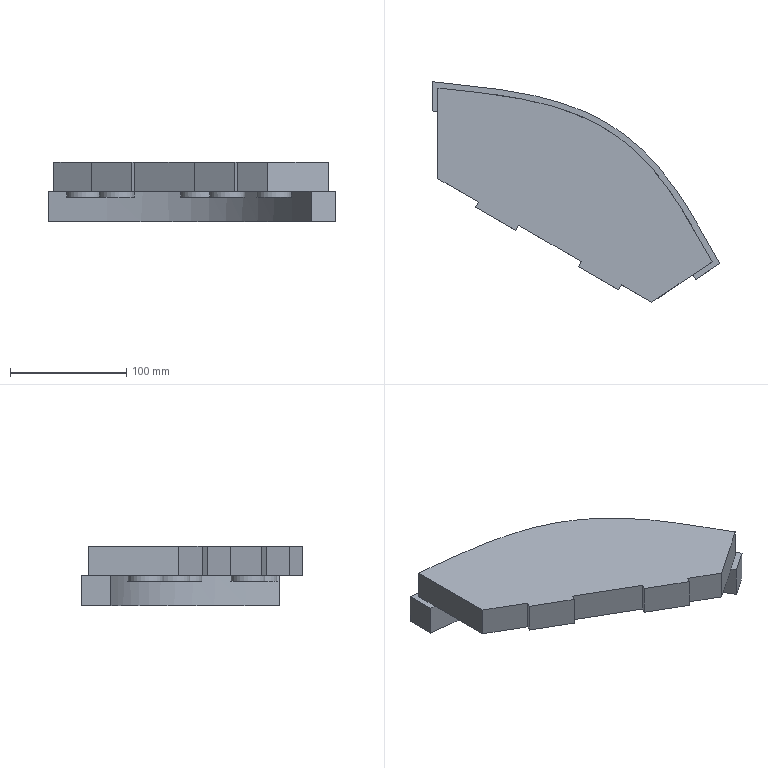Part | NX | features solid 2 | 1 solid | 30 faces | box 247.537 x 189.834 x 51 mm | volume 812442 mm3 | plane 22 | cylinder 5 | spline 3 | commonest cylinder face diameters 30 x5
STEP:
#1=CARTESIAN_POINT('',(-320.,-259.481,20.));
#2=VERTEX_POINT('',#1);
#3=CARTESIAN_POINT('',(-320.,-239.371,20.));
#4=VERTEX_POINT('',#3);
#5=CARTESIAN_POINT('',(-320.,-348.688,20.));
#6=DIRECTION('',(0.,1.,0.));
#7=VECTOR('',#6,1000.);
#8=LINE('',#5,#7);
#9=EDGE_CURVE('',#2,#4,#8,.T.);
#10=ORIENTED_EDGE('',*,*,#9,.T.);
#11=CARTESIAN_POINT('',(-84.106,-388.69,20.));
#12=VERTEX_POINT('',#11);
#13=CARTESIAN_POINT('',(-320.,-239.371,20.));
#14=CARTESIAN_POINT('',(-307.444,-240.685,20.));
#15=CARTESIAN_POINT('',(-282.388,-243.232,20.));
#16=CARTESIAN_POINT('',(-245.249,-248.591,20.));
#17=CARTESIAN_POINT('',(-209.143,-257.743,20.));
#18=CARTESIAN_POINT('',(-175.405,-272.915,20.));
#19=CARTESIAN_POINT('',(-146.181,-295.434,20.));
#20=CARTESIAN_POINT('',(-122.393,-323.908,20.));
#21=CARTESIAN_POINT('',(-102.621,-355.678,20.));
#22=CARTESIAN_POINT('',(-90.362,-377.698,20.));
#23=CARTESIAN_POINT('',(-84.106,-388.69,20.));
#24=B_SPLINE_CURVE_WITH_KNOTS('',3,(#13,#14,#15,#16,#17,#18,#19,#20,#21,#22,#23),.UNSPECIFIED.,.F.,.F.,(4,1,1,1,1,1,1,1,4),(0.01774,0.1387,0.2596,0.3805,0.5015,0.6224,0.7433,0.8643,0.9852),.UNSPECIFIED.);
#25=EDGE_CURVE('',#4,#12,#24,.T.);
#26=ORIENTED_EDGE('',*,*,#25,.T.);
#27=CARTESIAN_POINT('',(-100.733,-399.906,20.));
#28=VERTEX_POINT('',#27);
#29=CARTESIAN_POINT('',(-108.761,-405.32,20.));
#30=DIRECTION('',(-0.829,-0.5592,0.));
#31=VECTOR('',#30,1000.);
#32=LINE('',#29,#31);
#33=EDGE_CURVE('',#12,#28,#32,.T.);
#34=ORIENTED_EDGE('',*,*,#33,.T.);
#35=CARTESIAN_POINT('',(-98.242,-404.256,20.));
#36=VERTEX_POINT('',#35);
#37=CARTESIAN_POINT('',(-325.,-258.957,20.));
#38=CARTESIAN_POINT('',(-316.722,-259.827,20.));
#39=CARTESIAN_POINT('',(-294.324,-262.123,20.));
#40=CARTESIAN_POINT('',(-258.889,-266.42,20.));
#41=CARTESIAN_POINT('',(-226.806,-273.525,20.));
#42=CARTESIAN_POINT('',(-203.149,-282.324,20.));
#43=CARTESIAN_POINT('',(-186.806,-290.617,20.));
#44=CARTESIAN_POINT('',(-171.788,-300.874,20.));
#45=CARTESIAN_POINT('',(-158.202,-313.043,20.));
#46=CARTESIAN_POINT('',(-145.734,-327.185,20.));
#47=CARTESIAN_POINT('',(-130.501,-348.116,20.));
#48=CARTESIAN_POINT('',(-116.6,-371.801,20.));
#49=CARTESIAN_POINT('',(-104.721,-392.924,20.));
#50=CARTESIAN_POINT('',(-99.69,-401.736,20.));
#51=CARTESIAN_POINT('',(-98.242,-404.256,20.));
#52=B_SPLINE_CURVE_WITH_KNOTS('',3,(#37,#38,#39,#40,#41,#42,#43,#44,#45,#46,#47,#48,#49,#50,#51),.UNSPECIFIED.,.F.,.F.,(4,1,1,1,1,1,1,1,1,1,1,1,4),(0.,0.07955,0.2169,0.3543,0.423,0.4917,0.5604,0.6291,0.6978,0.7665,0.9039,0.9726,1.),.UNSPECIFIED.);
#53=EDGE_CURVE('',#36,#28,#52,.F.);
#54=ORIENTED_EDGE('',*,*,#53,.F.);
#55=CARTESIAN_POINT('',(-77.463,-390.241,20.));
#56=VERTEX_POINT('',#55);
#57=CARTESIAN_POINT('',(-98.242,-404.256,20.));
#58=DIRECTION('',(-0.829,-0.5592,0.));
#59=VECTOR('',#58,1000.);
#60=LINE('',#57,#59);
#61=EDGE_CURVE('',#56,#36,#60,.T.);
#62=ORIENTED_EDGE('',*,*,#61,.F.);
#63=CARTESIAN_POINT('',(-325.,-233.817,20.));
#64=VERTEX_POINT('',#63);
#65=CARTESIAN_POINT('',(-325.,-233.817,20.));
#66=CARTESIAN_POINT('',(-317.55,-234.605,20.));
#67=CARTESIAN_POINT('',(-296.291,-236.79,20.));
#68=CARTESIAN_POINT('',(-261.264,-240.795,20.));
#69=CARTESIAN_POINT('',(-220.344,-248.886,20.));
#70=CARTESIAN_POINT('',(-187.701,-261.197,20.));
#71=CARTESIAN_POINT('',(-163.887,-275.581,20.));
#72=CARTESIAN_POINT('',(-147.555,-288.567,20.));
#73=CARTESIAN_POINT('',(-132.971,-303.448,20.));
#74=CARTESIAN_POINT('',(-115.628,-325.186,20.));
#75=CARTESIAN_POINT('',(-97.505,-354.461,20.));
#76=CARTESIAN_POINT('',(-84.207,-378.469,20.));
#77=CARTESIAN_POINT('',(-77.463,-390.241,20.));
#78=B_SPLINE_CURVE_WITH_KNOTS('',3,(#65,#66,#67,#68,#69,#70,#71,#72,#73,#74,#75,#76,#77),.UNSPECIFIED.,.F.,.F.,(4,1,1,1,1,1,1,1,1,1,4),(0.,0.0718,0.2048,0.3379,0.4709,0.5374,0.6039,0.6704,0.7369,0.87,1.),.UNSPECIFIED.);
#79=EDGE_CURVE('',#56,#64,#78,.F.);
#80=ORIENTED_EDGE('',*,*,#79,.T.);
#81=CARTESIAN_POINT('',(-325.,-258.957,20.));
#82=VERTEX_POINT('',#81);
#83=CARTESIAN_POINT('',(-325.,-401.561,20.));
#84=DIRECTION('',(0.,1.,0.));
#85=VECTOR('',#84,1000.);
#86=LINE('',#83,#85);
#87=EDGE_CURVE('',#64,#82,#86,.F.);
#88=ORIENTED_EDGE('',*,*,#87,.T.);
#89=CARTESIAN_POINT('',(-325.,-258.957,20.));
#90=CARTESIAN_POINT('',(-316.722,-259.827,20.));
#91=CARTESIAN_POINT('',(-294.324,-262.123,20.));
#92=CARTESIAN_POINT('',(-258.889,-266.42,20.));
#93=CARTESIAN_POINT('',(-226.806,-273.525,20.));
#94=CARTESIAN_POINT('',(-203.149,-282.324,20.));
#95=CARTESIAN_POINT('',(-186.806,-290.617,20.));
#96=CARTESIAN_POINT('',(-171.788,-300.874,20.));
#97=CARTESIAN_POINT('',(-158.202,-313.043,20.));
#98=CARTESIAN_POINT('',(-145.734,-327.185,20.));
#99=CARTESIAN_POINT('',(-130.501,-348.116,20.));
#100=CARTESIAN_POINT('',(-116.6,-371.801,20.));
#101=CARTESIAN_POINT('',(-104.721,-392.924,20.));
#102=CARTESIAN_POINT('',(-99.69,-401.736,20.));
#103=CARTESIAN_POINT('',(-98.242,-404.256,20.));
#104=B_SPLINE_CURVE_WITH_KNOTS('',3,(#89,#90,#91,#92,#93,#94,#95,#96,#97,#98,#99,#100,#101,#102,#103),.UNSPECIFIED.,.F.,.F.,(4,1,1,1,1,1,1,1,1,1,1,1,4),(0.,0.07955,0.2169,0.3543,0.423,0.4917,0.5604,0.6291,0.6978,0.7665,0.9039,0.9726,1.),.UNSPECIFIED.);
#105=EDGE_CURVE('',#2,#82,#104,.F.);
#106=ORIENTED_EDGE('',*,*,#105,.F.);
#107=EDGE_LOOP('',(#10,#26,#34,#54,#62,#80,#88,#106));
#108=FACE_BOUND('',#107,.T.);
#109=CARTESIAN_POINT('',(-53.05,-401.561,20.));
#110=DIRECTION('',(0.,0.,1.));
#111=DIRECTION('',(1.,0.,0.));
#112=AXIS2_PLACEMENT_3D('',#109,#110,#111);
#113=PLANE('',#112);
#114=ADVANCED_FACE('',(#108),#113,.T.);
#115=CARTESIAN_POINT('',(-145.838,-387.024,20.));
#116=VERTEX_POINT('',#115);
#117=CARTESIAN_POINT('',(-130.838,-387.024,20.));
#118=DIRECTION('',(0.,0.,-1.));
#119=DIRECTION('',(-1.,0.,0.));
#120=AXIS2_PLACEMENT_3D('',#117,#118,#119);
#121=CIRCLE('',#120,15.);
#122=EDGE_CURVE('',#116,#116,#121,.T.);
#123=ORIENTED_EDGE('',*,*,#122,.T.);
#124=EDGE_LOOP('',(#123));
#125=FACE_BOUND('',#124,.T.);
#126=CARTESIAN_POINT('',(-115.838,-387.024,15.));
#127=VERTEX_POINT('',#126);
#128=CARTESIAN_POINT('',(-130.838,-387.024,15.));
#129=DIRECTION('',(0.,0.,1.));
#130=DIRECTION('',(1.,0.,0.));
#131=AXIS2_PLACEMENT_3D('',#128,#129,#130);
#132=CIRCLE('',#131,15.);
#133=EDGE_CURVE('',#127,#127,#132,.T.);
#134=ORIENTED_EDGE('',*,*,#133,.T.);
#135=EDGE_LOOP('',(#134));
#136=FACE_BOUND('',#135,.T.);
#137=CARTESIAN_POINT('',(-130.838,-387.024,20.));
#138=DIRECTION('',(0.,0.,-1.));
#139=DIRECTION('',(-0.866,-0.5,0.));
#140=AXIS2_PLACEMENT_3D('',#137,#138,#139);
#141=CYLINDRICAL_SURFACE('',#140,15.);
#142=ADVANCED_FACE('',(#125,#136),#141,.T.);
#143=CARTESIAN_POINT('',(-185.838,-377.024,20.));
#144=VERTEX_POINT('',#143);
#145=CARTESIAN_POINT('',(-170.838,-377.024,20.));
#146=DIRECTION('',(0.,0.,-1.));
#147=DIRECTION('',(-1.,0.,0.));
#148=AXIS2_PLACEMENT_3D('',#145,#146,#147);
#149=CIRCLE('',#148,15.);
#150=EDGE_CURVE('',#144,#144,#149,.T.);
#151=ORIENTED_EDGE('',*,*,#150,.T.);
#152=EDGE_LOOP('',(#151));
#153=FACE_BOUND('',#152,.T.);
#154=CARTESIAN_POINT('',(-157.848,-369.524,15.));
#155=VERTEX_POINT('',#154);
#156=CARTESIAN_POINT('',(-170.838,-377.024,15.));
#157=DIRECTION('',(0.,0.,-1.));
#158=DIRECTION('',(0.866,0.5,0.));
#159=AXIS2_PLACEMENT_3D('',#156,#157,#158);
#160=CIRCLE('',#159,15.);
#161=EDGE_CURVE('',#155,#155,#160,.T.);
#162=ORIENTED_EDGE('',*,*,#161,.F.);
#163=EDGE_LOOP('',(#162));
#164=FACE_BOUND('',#163,.T.);
#165=CARTESIAN_POINT('',(-170.838,-377.024,20.));
#166=DIRECTION('',(0.,0.,-1.));
#167=DIRECTION('',(-0.866,-0.5,0.));
#168=AXIS2_PLACEMENT_3D('',#165,#166,#167);
#169=CYLINDRICAL_SURFACE('',#168,15.);
#170=ADVANCED_FACE('',(#153,#164),#169,.T.);
#171=CARTESIAN_POINT('',(-325.,-258.957,-6.));
#172=VERTEX_POINT('',#171);
#173=CARTESIAN_POINT('',(-325.,-233.817,-6.));
#174=VERTEX_POINT('',#173);
#175=CARTESIAN_POINT('',(-325.,-258.957,-6.));
#176=DIRECTION('',(0.,1.,0.));
#177=VECTOR('',#176,1000.);
#178=LINE('',#175,#177);
#179=EDGE_CURVE('',#172,#174,#178,.T.);
#180=ORIENTED_EDGE('',*,*,#179,.F.);
#181=CARTESIAN_POINT('',(-325.,-258.957,45.));
#182=DIRECTION('',(0.,0.,-1.));
#183=VECTOR('',#182,1000.);
#184=LINE('',#181,#183);
#185=EDGE_CURVE('',#82,#172,#184,.T.);
#186=ORIENTED_EDGE('',*,*,#185,.F.);
#187=ORIENTED_EDGE('',*,*,#87,.F.);
#188=CARTESIAN_POINT('',(-325.,-233.817,45.));
#189=DIRECTION('',(0.,0.,-1.));
#190=VECTOR('',#189,1000.);
#191=LINE('',#188,#190);
#192=EDGE_CURVE('',#64,#174,#191,.T.);
#193=ORIENTED_EDGE('',*,*,#192,.T.);
#194=EDGE_LOOP('',(#180,#186,#187,#193));
#195=FACE_BOUND('',#194,.T.);
#196=CARTESIAN_POINT('',(-325.,-560.,0.));
#197=DIRECTION('',(1.,0.,0.));
#198=DIRECTION('',(0.,0.,-1.));
#199=AXIS2_PLACEMENT_3D('',#196,#197,#198);
#200=PLANE('',#199);
#201=ADVANCED_FACE('',(#195),#200,.F.);
#202=CARTESIAN_POINT('',(-77.463,-390.241,-6.));
#203=VERTEX_POINT('',#202);
#204=CARTESIAN_POINT('',(-325.,-233.817,-6.));
#205=CARTESIAN_POINT('',(-317.55,-234.605,-6.));
#206=CARTESIAN_POINT('',(-296.291,-236.79,-6.));
#207=CARTESIAN_POINT('',(-261.264,-240.795,-6.));
#208=CARTESIAN_POINT('',(-220.344,-248.886,-6.));
#209=CARTESIAN_POINT('',(-187.701,-261.197,-6.));
#210=CARTESIAN_POINT('',(-163.887,-275.581,-6.));
#211=CARTESIAN_POINT('',(-147.555,-288.567,-6.));
#212=CARTESIAN_POINT('',(-132.971,-303.448,-6.));
#213=CARTESIAN_POINT('',(-115.628,-325.186,-6.));
#214=CARTESIAN_POINT('',(-97.505,-354.461,-6.));
#215=CARTESIAN_POINT('',(-84.207,-378.469,-6.));
#216=CARTESIAN_POINT('',(-77.463,-390.241,-6.));
#217=B_SPLINE_CURVE_WITH_KNOTS('',3,(#204,#205,#206,#207,#208,#209,#210,#211,#212,#213,#214,#215,#216),.UNSPECIFIED.,.F.,.F.,(4,1,1,1,1,1,1,1,1,1,4),(0.,0.0718,0.2048,0.3379,0.4709,0.5374,0.6039,0.6704,0.7369,0.87,1.),.UNSPECIFIED.);
#218=EDGE_CURVE('',#174,#203,#217,.T.);
#219=ORIENTED_EDGE('',*,*,#218,.T.);
#220=CARTESIAN_POINT('',(-98.242,-404.256,-6.));
#221=VERTEX_POINT('',#220);
#222=CARTESIAN_POINT('',(-98.242,-404.256,-6.));
#223=DIRECTION('',(0.829,0.5592,0.));
#224=VECTOR('',#223,1000.);
#225=LINE('',#222,#224);
#226=EDGE_CURVE('',#221,#203,#225,.T.);
#227=ORIENTED_EDGE('',*,*,#226,.F.);
#228=CARTESIAN_POINT('',(-325.,-258.957,-6.));
#229=CARTESIAN_POINT('',(-316.722,-259.827,-6.));
#230=CARTESIAN_POINT('',(-294.324,-262.123,-6.));
#231=CARTESIAN_POINT('',(-258.889,-266.42,-6.));
#232=CARTESIAN_POINT('',(-226.806,-273.525,-6.));
#233=CARTESIAN_POINT('',(-203.149,-282.324,-6.));
#234=CARTESIAN_POINT('',(-186.806,-290.617,-6.));
#235=CARTESIAN_POINT('',(-171.788,-300.874,-6.));
#236=CARTESIAN_POINT('',(-158.202,-313.043,-6.));
#237=CARTESIAN_POINT('',(-145.734,-327.185,-6.));
#238=CARTESIAN_POINT('',(-130.501,-348.116,-6.));
#239=CARTESIAN_POINT('',(-116.6,-371.801,-6.));
#240=CARTESIAN_POINT('',(-104.721,-392.924,-6.));
#241=CARTESIAN_POINT('',(-99.69,-401.736,-6.));
#242=CARTESIAN_POINT('',(-98.242,-404.256,-6.));
#243=B_SPLINE_CURVE_WITH_KNOTS('',3,(#228,#229,#230,#231,#232,#233,#234,#235,#236,#237,#238,#239,#240,#241,#242),.UNSPECIFIED.,.F.,.F.,(4,1,1,1,1,1,1,1,1,1,1,1,4),(0.,0.07955,0.2169,0.3543,0.423,0.4917,0.5604,0.6291,0.6978,0.7665,0.9039,0.9726,1.),.UNSPECIFIED.);
#244=EDGE_CURVE('',#172,#221,#243,.T.);
#245=ORIENTED_EDGE('',*,*,#244,.F.);
#246=ORIENTED_EDGE('',*,*,#179,.T.);
#247=EDGE_LOOP('',(#219,#227,#245,#246));
#248=FACE_BOUND('',#247,.T.);
#249=CARTESIAN_POINT('',(-582.311,-1052.635,-6.));
#250=DIRECTION('',(0.,0.,1.));
#251=DIRECTION('',(1.,0.,0.));
#252=AXIS2_PLACEMENT_3D('',#249,#250,#251);
#253=PLANE('',#252);
#254=ADVANCED_FACE('',(#248),#253,.F.);
#255=CARTESIAN_POINT('',(-280.838,-312.024,20.));
#256=VERTEX_POINT('',#255);
#257=CARTESIAN_POINT('',(-265.838,-312.024,20.));
#258=DIRECTION('',(0.,0.,-1.));
#259=DIRECTION('',(-1.,0.,0.));
#260=AXIS2_PLACEMENT_3D('',#257,#258,#259);
#261=CIRCLE('',#260,15.);
#262=EDGE_CURVE('',#256,#256,#261,.T.);
#263=ORIENTED_EDGE('',*,*,#262,.F.);
#264=EDGE_LOOP('',(#263));
#265=FACE_BOUND('',#264,.T.);
#266=ORIENTED_EDGE('',*,*,#122,.F.);
#267=EDGE_LOOP('',(#266));
#268=FACE_BOUND('',#267,.T.);
#269=CARTESIAN_POINT('',(-309.188,-288.543,20.));
#270=VERTEX_POINT('',#269);
#271=CARTESIAN_POINT('',(-294.188,-288.543,20.));
#272=DIRECTION('',(0.,0.,-1.));
#273=DIRECTION('',(-1.,0.,0.));
#274=AXIS2_PLACEMENT_3D('',#271,#272,#273);
#275=CIRCLE('',#274,15.);
#276=EDGE_CURVE('',#270,#270,#275,.T.);
#277=ORIENTED_EDGE('',*,*,#276,.F.);
#278=EDGE_LOOP('',(#277));
#279=FACE_BOUND('',#278,.T.);
#280=CARTESIAN_POINT('',(-210.838,-322.024,20.));
#281=VERTEX_POINT('',#280);
#282=CARTESIAN_POINT('',(-195.838,-322.024,20.));
#283=DIRECTION('',(0.,0.,-1.));
#284=DIRECTION('',(-1.,0.,0.));
#285=AXIS2_PLACEMENT_3D('',#282,#283,#284);
#286=CIRCLE('',#285,15.);
#287=EDGE_CURVE('',#281,#281,#286,.T.);
#288=ORIENTED_EDGE('',*,*,#287,.F.);
#289=EDGE_LOOP('',(#288));
#290=FACE_BOUND('',#289,.T.);
#291=CARTESIAN_POINT('',(-320.,-259.481,20.));
#292=CARTESIAN_POINT('',(-308.475,-260.684,20.));
#293=CARTESIAN_POINT('',(-285.416,-263.051,20.));
#294=CARTESIAN_POINT('',(-251.082,-267.927,20.));
#295=CARTESIAN_POINT('',(-222.914,-274.771,20.));
#296=CARTESIAN_POINT('',(-201.046,-283.292,20.));
#297=CARTESIAN_POINT('',(-185.448,-291.461,20.));
#298=CARTESIAN_POINT('',(-171.129,-301.443,20.));
#299=CARTESIAN_POINT('',(-154.042,-316.84,20.));
#300=CARTESIAN_POINT('',(-135.792,-339.802,20.));
#301=CARTESIAN_POINT('',(-117.789,-369.539,20.));
#302=CARTESIAN_POINT('',(-106.486,-389.828,20.));
#303=CARTESIAN_POINT('',(-100.733,-399.906,20.));
#304=B_SPLINE_CURVE_WITH_KNOTS('',3,(#291,#292,#293,#294,#295,#296,#297,#298,#299,#300,#301,#302,#303),.UNSPECIFIED.,.F.,.F.,(4,1,1,1,1,1,1,1,1,1,4),(0.6352,0.6699,0.7047,0.7394,0.7568,0.7742,0.7916,0.809,0.8437,0.8785,0.9133),.UNSPECIFIED.);
#305=EDGE_CURVE('',#2,#28,#304,.T.);
#306=ORIENTED_EDGE('',*,*,#305,.T.);
#307=CARTESIAN_POINT('',(-135.938,-423.652,20.));
#308=VERTEX_POINT('',#307);
#309=CARTESIAN_POINT('',(-108.761,-405.32,20.));
#310=DIRECTION('',(-0.829,-0.5592,0.));
#311=VECTOR('',#310,1000.);
#312=LINE('',#309,#311);
#313=EDGE_CURVE('',#28,#308,#312,.T.);
#314=ORIENTED_EDGE('',*,*,#313,.T.);
#315=CARTESIAN_POINT('',(-161.919,-408.652,20.));
#316=VERTEX_POINT('',#315);
#317=CARTESIAN_POINT('',(-229.815,-369.451,20.));
#318=DIRECTION('',(-0.866,0.5,0.));
#319=VECTOR('',#318,1000.);
#320=LINE('',#317,#319);
#321=EDGE_CURVE('',#308,#316,#320,.T.);
#322=ORIENTED_EDGE('',*,*,#321,.T.);
#323=CARTESIAN_POINT('',(-164.419,-412.982,20.));
#324=VERTEX_POINT('',#323);
#325=CARTESIAN_POINT('',(-164.419,-412.982,20.));
#326=DIRECTION('',(0.5,0.866,0.));
#327=VECTOR('',#326,1000.);
#328=LINE('',#325,#327);
#329=EDGE_CURVE('',#324,#316,#328,.T.);
#330=ORIENTED_EDGE('',*,*,#329,.F.);
#331=CARTESIAN_POINT('',(-199.06,-392.982,20.));
#332=VERTEX_POINT('',#331);
#333=CARTESIAN_POINT('',(-108.875,-445.05,20.));
#334=DIRECTION('',(-0.866,0.5,0.));
#335=VECTOR('',#334,1000.);
#336=LINE('',#333,#335);
#337=EDGE_CURVE('',#324,#332,#336,.T.);
#338=ORIENTED_EDGE('',*,*,#337,.T.);
#339=CARTESIAN_POINT('',(-196.56,-388.652,20.));
#340=VERTEX_POINT('',#339);
#341=CARTESIAN_POINT('',(-199.06,-392.982,20.));
#342=DIRECTION('',(0.5,0.866,0.));
#343=VECTOR('',#342,1000.);
#344=LINE('',#341,#343);
#345=EDGE_CURVE('',#332,#340,#344,.T.);
#346=ORIENTED_EDGE('',*,*,#345,.T.);
#347=CARTESIAN_POINT('',(-250.718,-357.383,20.));
#348=VERTEX_POINT('',#347);
#349=CARTESIAN_POINT('',(-229.815,-369.451,20.));
#350=DIRECTION('',(-0.866,0.5,0.));
#351=VECTOR('',#350,1000.);
#352=LINE('',#349,#351);
#353=EDGE_CURVE('',#340,#348,#352,.T.);
#354=ORIENTED_EDGE('',*,*,#353,.T.);
#355=CARTESIAN_POINT('',(-253.218,-361.713,20.));
#356=VERTEX_POINT('',#355);
#357=CARTESIAN_POINT('',(-253.218,-361.713,20.));
#358=DIRECTION('',(-0.5,-0.866,0.));
#359=VECTOR('',#358,1000.);
#360=LINE('',#357,#359);
#361=EDGE_CURVE('',#356,#348,#360,.F.);
#362=ORIENTED_EDGE('',*,*,#361,.F.);
#363=CARTESIAN_POINT('',(-287.859,-341.713,20.));
#364=VERTEX_POINT('',#363);
#365=CARTESIAN_POINT('',(-232.315,-373.782,20.));
#366=DIRECTION('',(-0.866,0.5,0.));
#367=VECTOR('',#366,1000.);
#368=LINE('',#365,#367);
#369=EDGE_CURVE('',#356,#364,#368,.T.);
#370=ORIENTED_EDGE('',*,*,#369,.T.);
#371=CARTESIAN_POINT('',(-285.359,-337.383,20.));
#372=VERTEX_POINT('',#371);
#373=CARTESIAN_POINT('',(-287.859,-341.713,20.));
#374=DIRECTION('',(-0.5,-0.866,0.));
#375=VECTOR('',#374,1000.);
#376=LINE('',#373,#375);
#377=EDGE_CURVE('',#364,#372,#376,.F.);
#378=ORIENTED_EDGE('',*,*,#377,.T.);
#379=CARTESIAN_POINT('',(-320.,-317.383,20.));
#380=VERTEX_POINT('',#379);
#381=CARTESIAN_POINT('',(-229.815,-369.451,20.));
#382=DIRECTION('',(-0.866,0.5,0.));
#383=VECTOR('',#382,1000.);
#384=LINE('',#381,#383);
#385=EDGE_CURVE('',#372,#380,#384,.T.);
#386=ORIENTED_EDGE('',*,*,#385,.T.);
#387=CARTESIAN_POINT('',(-320.,-348.688,20.));
#388=DIRECTION('',(0.,1.,0.));
#389=VECTOR('',#388,1000.);
#390=LINE('',#387,#389);
#391=EDGE_CURVE('',#380,#2,#390,.T.);
#392=ORIENTED_EDGE('',*,*,#391,.T.);
#393=EDGE_LOOP('',(#306,#314,#322,#330,#338,#346,#354,#362,#370,#378,#386,#392));
#394=FACE_BOUND('',#393,.T.);
#395=ORIENTED_EDGE('',*,*,#150,.F.);
#396=EDGE_LOOP('',(#395));
#397=FACE_BOUND('',#396,.T.);
#398=CARTESIAN_POINT('',(-53.05,-401.561,20.));
#399=DIRECTION('',(0.,0.,-1.));
#400=DIRECTION('',(-1.,0.,0.));
#401=AXIS2_PLACEMENT_3D('',#398,#399,#400);
#402=PLANE('',#401);
#403=ADVANCED_FACE('',(#265,#268,#279,#290,#394,#397),#402,.T.);
#404=CARTESIAN_POINT('',(-320.,-317.383,45.));
#405=VERTEX_POINT('',#404);
#406=CARTESIAN_POINT('',(-320.,-239.371,45.));
#407=VERTEX_POINT('',#406);
#408=CARTESIAN_POINT('',(-320.,-348.688,45.));
#409=DIRECTION('',(0.,1.,0.));
#410=VECTOR('',#409,1000.);
#411=LINE('',#408,#410);
#412=EDGE_CURVE('',#405,#407,#411,.T.);
#413=ORIENTED_EDGE('',*,*,#412,.F.);
#414=CARTESIAN_POINT('',(-285.359,-337.383,45.));
#415=VERTEX_POINT('',#414);
#416=CARTESIAN_POINT('',(-131.12,-426.433,45.));
#417=DIRECTION('',(-0.866,0.5,0.));
#418=VECTOR('',#417,1000.);
#419=LINE('',#416,#418);
#420=EDGE_CURVE('',#415,#405,#419,.T.);
#421=ORIENTED_EDGE('',*,*,#420,.F.);
#422=CARTESIAN_POINT('',(-287.859,-341.713,45.));
#423=VERTEX_POINT('',#422);
#424=CARTESIAN_POINT('',(-287.859,-341.713,45.));
#425=DIRECTION('',(0.5,0.866,0.));
#426=VECTOR('',#425,1000.);
#427=LINE('',#424,#426);
#428=EDGE_CURVE('',#423,#415,#427,.T.);
#429=ORIENTED_EDGE('',*,*,#428,.F.);
#430=CARTESIAN_POINT('',(-253.218,-361.713,45.));
#431=VERTEX_POINT('',#430);
#432=CARTESIAN_POINT('',(-133.62,-430.763,45.));
#433=DIRECTION('',(-0.866,0.5,0.));
#434=VECTOR('',#433,1000.);
#435=LINE('',#432,#434);
#436=EDGE_CURVE('',#431,#423,#435,.T.);
#437=ORIENTED_EDGE('',*,*,#436,.F.);
#438=CARTESIAN_POINT('',(-250.718,-357.383,45.));
#439=VERTEX_POINT('',#438);
#440=CARTESIAN_POINT('',(-253.218,-361.713,45.));
#441=DIRECTION('',(0.5,0.866,0.));
#442=VECTOR('',#441,1000.);
#443=LINE('',#440,#442);
#444=EDGE_CURVE('',#431,#439,#443,.T.);
#445=ORIENTED_EDGE('',*,*,#444,.T.);
#446=CARTESIAN_POINT('',(-196.56,-388.652,45.));
#447=VERTEX_POINT('',#446);
#448=CARTESIAN_POINT('',(-131.12,-426.433,45.));
#449=DIRECTION('',(-0.866,0.5,0.));
#450=VECTOR('',#449,1000.);
#451=LINE('',#448,#450);
#452=EDGE_CURVE('',#447,#439,#451,.T.);
#453=ORIENTED_EDGE('',*,*,#452,.F.);
#454=CARTESIAN_POINT('',(-199.06,-392.982,45.));
#455=VERTEX_POINT('',#454);
#456=CARTESIAN_POINT('',(-199.06,-392.982,45.));
#457=DIRECTION('',(0.5,0.866,0.));
#458=VECTOR('',#457,1000.);
#459=LINE('',#456,#458);
#460=EDGE_CURVE('',#455,#447,#459,.T.);
#461=ORIENTED_EDGE('',*,*,#460,.F.);
#462=CARTESIAN_POINT('',(-164.419,-412.982,45.));
#463=VERTEX_POINT('',#462);
#464=CARTESIAN_POINT('',(-10.18,-502.032,45.));
#465=DIRECTION('',(-0.866,0.5,0.));
#466=VECTOR('',#465,1000.);
#467=LINE('',#464,#466);
#468=EDGE_CURVE('',#463,#455,#467,.T.);
#469=ORIENTED_EDGE('',*,*,#468,.F.);
#470=CARTESIAN_POINT('',(-161.919,-408.652,45.));
#471=VERTEX_POINT('',#470);
#472=CARTESIAN_POINT('',(-164.419,-412.982,45.));
#473=DIRECTION('',(0.5,0.866,0.));
#474=VECTOR('',#473,1000.);
#475=LINE('',#472,#474);
#476=EDGE_CURVE('',#463,#471,#475,.T.);
#477=ORIENTED_EDGE('',*,*,#476,.T.);
#478=CARTESIAN_POINT('',(-135.938,-423.652,45.));
#479=VERTEX_POINT('',#478);
#480=CARTESIAN_POINT('',(-131.12,-426.433,45.));
#481=DIRECTION('',(-0.866,0.5,0.));
#482=VECTOR('',#481,1000.);
#483=LINE('',#480,#482);
#484=EDGE_CURVE('',#479,#471,#483,.T.);
#485=ORIENTED_EDGE('',*,*,#484,.F.);
#486=CARTESIAN_POINT('',(-84.106,-388.69,45.));
#487=VERTEX_POINT('',#486);
#488=CARTESIAN_POINT('',(-108.761,-405.32,45.));
#489=DIRECTION('',(-0.829,-0.5592,0.));
#490=VECTOR('',#489,1000.);
#491=LINE('',#488,#490);
#492=EDGE_CURVE('',#487,#479,#491,.T.);
#493=ORIENTED_EDGE('',*,*,#492,.F.);
#494=CARTESIAN_POINT('',(-84.106,-388.69,45.));
#495=CARTESIAN_POINT('',(-85.647,-385.982,45.));
#496=CARTESIAN_POINT('',(-88.727,-380.563,45.));
#497=CARTESIAN_POINT('',(-92.552,-373.785,45.));
#498=CARTESIAN_POINT('',(-95.629,-368.349,45.));
#499=CARTESIAN_POINT('',(-97.957,-364.289,45.));
#500=CARTESIAN_POINT('',(-99.9,-360.932,45.));
#501=CARTESIAN_POINT('',(-101.482,-358.221,45.));
#502=CARTESIAN_POINT('',(-102.617,-356.285,45.));
#503=CARTESIAN_POINT('',(-103.968,-353.996,45.));
#504=CARTESIAN_POINT('',(-105.653,-351.166,45.));
#505=CARTESIAN_POINT('',(-107.726,-347.73,45.));
#506=CARTESIAN_POINT('',(-109.714,-344.499,45.));
#507=CARTESIAN_POINT('',(-111.054,-342.356,45.));
#508=CARTESIAN_POINT('',(-111.826,-341.133,45.));
#509=CARTESIAN_POINT('',(-112.348,-340.31,45.));
#510=CARTESIAN_POINT('',(-113.056,-339.2,45.));
#511=CARTESIAN_POINT('',(-113.932,-337.837,45.));
#512=CARTESIAN_POINT('',(-115.49,-335.441,45.));
#513=CARTESIAN_POINT('',(-117.678,-332.15,45.));
#514=CARTESIAN_POINT('',(-119.851,-328.982,45.));
#515=CARTESIAN_POINT('',(-121.348,-326.852,45.));
#516=CARTESIAN_POINT('',(-122.214,-325.635,45.));
#517=CARTESIAN_POINT('',(-122.82,-324.791,45.));
#518=CARTESIAN_POINT('',(-123.584,-323.737,45.));
#519=CARTESIAN_POINT('',(-124.55,-322.418,45.));
#520=CARTESIAN_POINT('',(-126.27,-320.104,45.));
#521=CARTESIAN_POINT('',(-128.729,-316.899,45.));
#522=CARTESIAN_POINT('',(-131.71,-313.175,45.));
#523=CARTESIAN_POINT('',(-135.713,-308.387,45.));
#524=CARTESIAN_POINT('',(-139.769,-303.854,45.));
#525=CARTESIAN_POINT('',(-143.344,-300.132,45.));
#526=CARTESIAN_POINT('',(-145.423,-298.047,45.));
#527=CARTESIAN_POINT('',(-146.92,-296.581,45.));
#528=CARTESIAN_POINT('',(-148.681,-294.902,45.));
#529=CARTESIAN_POINT('',(-150.968,-292.786,45.));
#530=CARTESIAN_POINT('',(-155.076,-289.142,45.));
#531=CARTESIAN_POINT('',(-161.107,-284.243,45.));
#532=CARTESIAN_POINT('',(-167.411,-279.706,45.));
#533=CARTESIAN_POINT('',(-172.571,-276.323,45.));
#534=CARTESIAN_POINT('',(-176.604,-273.848,45.));
#535=CARTESIAN_POINT('',(-180.375,-271.68,45.));
#536=CARTESIAN_POINT('',(-185.668,-268.822,45.));
#537=CARTESIAN_POINT('',(-192.496,-265.486,45.));
#538=CARTESIAN_POINT('',(-199.688,-262.414,45.));
#539=CARTESIAN_POINT('',(-204.89,-260.415,45.));
#540=CARTESIAN_POINT('',(-207.551,-259.447,45.));
#541=CARTESIAN_POINT('',(-209.061,-258.912,45.));
#542=CARTESIAN_POINT('',(-210.265,-258.493,45.));
#543=CARTESIAN_POINT('',(-211.229,-258.164,45.));
#544=CARTESIAN_POINT('',(-212.61,-257.7,45.));
#545=CARTESIAN_POINT('',(-215.012,-256.913,45.));
#546=CARTESIAN_POINT('',(-219.945,-255.377,45.));
#547=CARTESIAN_POINT('',(-225.8,-253.731,45.));
#548=CARTESIAN_POINT('',(-231.888,-252.19,45.));
#549=CARTESIAN_POINT('',(-236.572,-251.087,45.));
#550=CARTESIAN_POINT('',(-240.558,-250.215,45.));
#551=CARTESIAN_POINT('',(-243.425,-249.623,45.));
#552=CARTESIAN_POINT('',(-245.035,-249.299,45.));
#553=CARTESIAN_POINT('',(-246.369,-249.037,45.));
#554=CARTESIAN_POINT('',(-247.258,-248.865,45.));
#555=CARTESIAN_POINT('',(-248.616,-248.606,45.));
#556=CARTESIAN_POINT('',(-250.955,-248.17,45.));
#557=CARTESIAN_POINT('',(-254.441,-247.55,45.));
#558=CARTESIAN_POINT('',(-258.776,-246.824,45.));
#559=CARTESIAN_POINT('',(-263.283,-246.113,45.));
#560=CARTESIAN_POINT('',(-267.958,-245.416,45.));
#561=CARTESIAN_POINT('',(-271.994,-244.849,45.));
#562=CARTESIAN_POINT('',(-275.306,-244.402,45.));
#563=CARTESIAN_POINT('',(-277.835,-244.071,45.));
#564=CARTESIAN_POINT('',(-279.969,-243.799,45.));
#565=CARTESIAN_POINT('',(-281.498,-243.608,45.));
#566=CARTESIAN_POINT('',(-282.35,-243.502,45.));
#567=CARTESIAN_POINT('',(-283.068,-243.414,45.));
#568=CARTESIAN_POINT('',(-283.497,-243.362,45.));
#569=CARTESIAN_POINT('',(-284.179,-243.279,45.));
#570=CARTESIAN_POINT('',(-285.345,-243.139,45.));
#571=CARTESIAN_POINT('',(-287.787,-242.849,45.));
#572=CARTESIAN_POINT('',(-290.744,-242.507,45.));
#573=CARTESIAN_POINT('',(-293.883,-242.153,45.));
#574=CARTESIAN_POINT('',(-295.92,-241.927,45.));
#575=CARTESIAN_POINT('',(-297.593,-241.742,45.));
#576=CARTESIAN_POINT('',(-298.874,-241.603,45.));
#577=CARTESIAN_POINT('',(-299.948,-241.486,45.));
#578=CARTESIAN_POINT('',(-300.732,-241.401,45.));
#579=CARTESIAN_POINT('',(-301.149,-241.356,45.));
#580=CARTESIAN_POINT('',(-301.559,-241.312,45.));
#581=CARTESIAN_POINT('',(-301.604,-241.307,45.));
#582=CARTESIAN_POINT('',(-301.8,-241.286,45.));
#583=CARTESIAN_POINT('',(-302.102,-241.254,45.));
#584=CARTESIAN_POINT('',(-302.617,-241.199,45.));
#585=CARTESIAN_POINT('',(-303.307,-241.126,45.));
#586=CARTESIAN_POINT('',(-304.343,-241.016,45.));
#587=CARTESIAN_POINT('',(-305.848,-240.857,45.));
#588=CARTESIAN_POINT('',(-308.707,-240.555,45.));
#589=CARTESIAN_POINT('',(-313.124,-240.091,45.));
#590=CARTESIAN_POINT('',(-317.558,-239.626,45.));
#591=CARTESIAN_POINT('',(-320.,-239.371,45.));
#592=B_SPLINE_CURVE_WITH_KNOTS('',3,(#494,#495,#496,#497,#498,#499,#500,#501,#502,#503,#504,#505,#506,#507,#508,#509,#510,#511,#512,#513,#514,#515,#516,#517,#518,#519,#520,#521,#522,#523,#524,#525,#526,#527,#528,#529,#530,#531,#532,#533,#534,#535,#536,#537,#538,#539,#540,#541,#542,#543,#544,#545,#546,#547,#548,#549,#550,#551,#552,#553,#554,#555,#556,#557,#558,#559,#560,#561,#562,#563,#564,#565,#566,#567,#568,#569,#570,#571,#572,#573,#574,#575,#576,#577,#578,#579,#580,#581,#582,#583,#584,#585,#586,#587,#588,#589,#590,#591),.UNSPECIFIED.,.F.,.F.,(4,1,1,1,1,1,1,1,1,1,1,1,1,1,1,1,1,1,1,1,1,1,1,1,1,1,1,1,1,1,1,1,1,1,1,1,1,1,1,1,1,1,1,1,1,1,1,1,1,1,1,1,1,1,1,1,1,1,1,1,1,1,1,1,1,1,1,1,1,1,1,1,1,1,1,1,1,1,1,1,1,1,1,1,1,1,1,1,1,1,1,1,1,1,1,4),(0.,0.03125,0.0625,0.07812,0.09375,0.1094,0.1172,0.125,0.1328,0.1406,0.1562,0.1719,0.1797,0.1836,0.1875,0.1914,0.1953,0.2031,0.2188,0.2344,0.2422,0.2461,0.25,0.2539,0.2578,0.2656,0.2812,0.2969,0.3125,0.3438,0.3594,0.3672,0.375,0.3828,0.3906,0.4062,0.4375,0.4688,0.4844,0.5,0.5156,0.5312,0.5625,0.5938,0.6094,0.6172,0.6211,0.625,0.6289,0.6328,0.6406,0.6562,0.6875,0.7031,0.7188,0.7344,0.7422,0.7461,0.75,0.7539,0.7578,0.7656,0.7812,0.7969,0.8125,0.8281,0.8438,0.8516,0.8594,0.8672,0.8711,0.873,0.875,0.877,0.8789,0.8828,0.8906,0.9062,0.9141,0.9219,0.9258,0.9297,0.9336,0.9355,0.9365,0.9375,0.9385,0.9395,0.9414,0.9453,0.9492,0.9531,0.9609,0.9688,0.9844,1.),.UNSPECIFIED.);
#593=EDGE_CURVE('',#487,#407,#592,.T.);
#594=ORIENTED_EDGE('',*,*,#593,.T.);
#595=EDGE_LOOP('',(#413,#421,#429,#437,#445,#453,#461,#469,#477,#485,#493,#594));
#596=FACE_BOUND('',#595,.T.);
#597=CARTESIAN_POINT('',(-582.311,-1052.635,45.));
#598=DIRECTION('',(0.,0.,1.));
#599=DIRECTION('',(1.,0.,0.));
#600=AXIS2_PLACEMENT_3D('',#597,#598,#599);
#601=PLANE('',#600);
#602=ADVANCED_FACE('',(#596),#601,.T.);
#603=ORIENTED_EDGE('',*,*,#133,.F.);
#604=EDGE_LOOP('',(#603));
#605=FACE_BOUND('',#604,.T.);
#606=CARTESIAN_POINT('',(-118.429,-400.345,15.));
#607=DIRECTION('',(0.,0.,1.));
#608=DIRECTION('',(1.,0.,0.));
#609=AXIS2_PLACEMENT_3D('',#606,#607,#608);
#610=PLANE('',#609);
#611=ADVANCED_FACE('',(#605),#610,.F.);
#612=ORIENTED_EDGE('',*,*,#391,.F.);
#613=CARTESIAN_POINT('',(-320.,-317.383,45.));
#614=DIRECTION('',(0.,0.,1.));
#615=VECTOR('',#614,1000.);
#616=LINE('',#613,#615);
#617=EDGE_CURVE('',#380,#405,#616,.T.);
#618=ORIENTED_EDGE('',*,*,#617,.T.);
#619=ORIENTED_EDGE('',*,*,#412,.T.);
#620=CARTESIAN_POINT('',(-320.,-239.371,32.5));
#621=DIRECTION('',(0.,0.,1.));
#622=VECTOR('',#621,1000.);
#623=LINE('',#620,#622);
#624=EDGE_CURVE('',#4,#407,#623,.T.);
#625=ORIENTED_EDGE('',*,*,#624,.F.);
#626=ORIENTED_EDGE('',*,*,#9,.F.);
#627=EDGE_LOOP('',(#612,#618,#619,#625,#626));
#628=FACE_BOUND('',#627,.T.);
#629=CARTESIAN_POINT('',(-320.,-348.688,45.));
#630=DIRECTION('',(-1.,0.,0.));
#631=DIRECTION('',(0.,0.,1.));
#632=AXIS2_PLACEMENT_3D('',#629,#630,#631);
#633=PLANE('',#632);
#634=ADVANCED_FACE('',(#628),#633,.T.);
#635=CARTESIAN_POINT('',(-250.838,-312.024,15.));
#636=VERTEX_POINT('',#635);
#637=CARTESIAN_POINT('',(-265.838,-312.024,15.));
#638=DIRECTION('',(0.,0.,1.));
#639=DIRECTION('',(1.,0.,0.));
#640=AXIS2_PLACEMENT_3D('',#637,#638,#639);
#641=CIRCLE('',#640,15.);
#642=EDGE_CURVE('',#636,#636,#641,.T.);
#643=ORIENTED_EDGE('',*,*,#642,.F.);
#644=EDGE_LOOP('',(#643));
#645=FACE_BOUND('',#644,.T.);
#646=CARTESIAN_POINT('',(-258.429,-320.345,15.));
#647=DIRECTION('',(0.,0.,1.));
#648=DIRECTION('',(1.,0.,0.));
#649=AXIS2_PLACEMENT_3D('',#646,#647,#648);
#650=PLANE('',#649);
#651=ADVANCED_FACE('',(#645),#650,.F.);
#652=CARTESIAN_POINT('',(-281.197,-281.043,15.));
#653=VERTEX_POINT('',#652);
#654=CARTESIAN_POINT('',(-294.188,-288.543,15.));
#655=DIRECTION('',(0.,0.,-1.));
#656=DIRECTION('',(0.866,0.5,0.));
#657=AXIS2_PLACEMENT_3D('',#654,#655,#656);
#658=CIRCLE('',#657,15.);
#659=EDGE_CURVE('',#653,#653,#658,.T.);
#660=ORIENTED_EDGE('',*,*,#659,.T.);
#661=EDGE_LOOP('',(#660));
#662=FACE_BOUND('',#661,.T.);
#663=CARTESIAN_POINT('',(-283.429,-300.345,15.));
#664=DIRECTION('',(0.,0.,1.));
#665=DIRECTION('',(1.,0.,0.));
#666=AXIS2_PLACEMENT_3D('',#663,#664,#665);
#667=PLANE('',#666);
#668=ADVANCED_FACE('',(#662),#667,.F.);
#669=ORIENTED_EDGE('',*,*,#161,.T.);
#670=EDGE_LOOP('',(#669));
#671=FACE_BOUND('',#670,.T.);
#672=CARTESIAN_POINT('',(-153.429,-395.345,15.));
#673=DIRECTION('',(0.,0.,1.));
#674=DIRECTION('',(1.,0.,0.));
#675=AXIS2_PLACEMENT_3D('',#672,#673,#674);
#676=PLANE('',#675);
#677=ADVANCED_FACE('',(#671),#676,.F.);
#678=ORIENTED_EDGE('',*,*,#262,.T.);
#679=EDGE_LOOP('',(#678));
#680=FACE_BOUND('',#679,.T.);
#681=ORIENTED_EDGE('',*,*,#642,.T.);
#682=EDGE_LOOP('',(#681));
#683=FACE_BOUND('',#682,.T.);
#684=CARTESIAN_POINT('',(-265.838,-312.024,20.));
#685=DIRECTION('',(0.,0.,-1.));
#686=DIRECTION('',(-0.866,-0.5,0.));
#687=AXIS2_PLACEMENT_3D('',#684,#685,#686);
#688=CYLINDRICAL_SURFACE('',#687,15.);
#689=ADVANCED_FACE('',(#680,#683),#688,.T.);
#690=CARTESIAN_POINT('',(-182.848,-314.524,15.));
#691=VERTEX_POINT('',#690);
#692=CARTESIAN_POINT('',(-195.838,-322.024,15.));
#693=DIRECTION('',(0.,0.,-1.));
#694=DIRECTION('',(0.866,0.5,0.));
#695=AXIS2_PLACEMENT_3D('',#692,#693,#694);
#696=CIRCLE('',#695,15.);
#697=EDGE_CURVE('',#691,#691,#696,.T.);
#698=ORIENTED_EDGE('',*,*,#697,.T.);
#699=EDGE_LOOP('',(#698));
#700=FACE_BOUND('',#699,.T.);
#701=CARTESIAN_POINT('',(-195.838,-322.024,15.));
#702=DIRECTION('',(0.,0.,-1.));
#703=DIRECTION('',(-0.866,-0.5,0.));
#704=AXIS2_PLACEMENT_3D('',#701,#702,#703);
#705=PLANE('',#704);
#706=ADVANCED_FACE('',(#700),#705,.T.);
#707=ORIENTED_EDGE('',*,*,#244,.T.);
#708=CARTESIAN_POINT('',(-98.242,-404.256,45.));
#709=DIRECTION('',(0.,0.,-1.));
#710=VECTOR('',#709,1000.);
#711=LINE('',#708,#710);
#712=EDGE_CURVE('',#36,#221,#711,.T.);
#713=ORIENTED_EDGE('',*,*,#712,.F.);
#714=ORIENTED_EDGE('',*,*,#53,.T.);
#715=ORIENTED_EDGE('',*,*,#305,.F.);
#716=ORIENTED_EDGE('',*,*,#105,.T.);
#717=ORIENTED_EDGE('',*,*,#185,.T.);
#718=EDGE_LOOP('',(#707,#713,#714,#715,#716,#717));
#719=FACE_BOUND('',#718,.T.);
#720=CARTESIAN_POINT('',(-325.,-258.957,20.));
#721=CARTESIAN_POINT('',(-325.,-258.957,-6.));
#722=CARTESIAN_POINT('',(-298.986,-261.69,20.));
#723=CARTESIAN_POINT('',(-298.986,-261.69,-6.));
#724=CARTESIAN_POINT('',(-260.913,-265.249,20.));
#725=CARTESIAN_POINT('',(-260.913,-265.249,-6.));
#726=CARTESIAN_POINT('',(-214.978,-276.918,20.));
#727=CARTESIAN_POINT('',(-214.978,-276.918,-6.));
#728=CARTESIAN_POINT('',(-184.347,-291.007,20.));
#729=CARTESIAN_POINT('',(-184.347,-291.007,-6.));
#730=CARTESIAN_POINT('',(-158.497,-311.525,20.));
#731=CARTESIAN_POINT('',(-158.497,-311.525,-6.));
#732=CARTESIAN_POINT('',(-136.666,-338.441,20.));
#733=CARTESIAN_POINT('',(-136.666,-338.441,-6.));
#734=CARTESIAN_POINT('',(-117.445,-370.042,20.));
#735=CARTESIAN_POINT('',(-117.445,-370.042,-6.));
#736=CARTESIAN_POINT('',(-104.839,-392.778,20.));
#737=CARTESIAN_POINT('',(-104.839,-392.778,-6.));
#738=CARTESIAN_POINT('',(-98.242,-404.256,20.));
#739=CARTESIAN_POINT('',(-98.242,-404.256,-6.));
#740=B_SPLINE_SURFACE_WITH_KNOTS('',3,1,((#720,#721),(#722,#723),(#724,#725),(#726,#727),(#728,#729),(#730,#731),(#732,#733),(#734,#735),(#736,#737),(#738,#739)),.SURF_OF_LINEAR_EXTRUSION.,.F.,.F.,.F.,(4,1,1,1,1,1,1,4),(2,2),(0.,0.25,0.375,0.5,0.625,0.75,0.875,1.),(0.,1.),.UNSPECIFIED.);
#741=ADVANCED_FACE('',(#719),#740,.F.);
#742=ORIENTED_EDGE('',*,*,#659,.F.);
#743=EDGE_LOOP('',(#742));
#744=FACE_BOUND('',#743,.T.);
#745=ORIENTED_EDGE('',*,*,#276,.T.);
#746=EDGE_LOOP('',(#745));
#747=FACE_BOUND('',#746,.T.);
#748=CARTESIAN_POINT('',(-294.188,-288.543,20.));
#749=DIRECTION('',(0.,0.,-1.));
#750=DIRECTION('',(-0.866,-0.5,0.));
#751=AXIS2_PLACEMENT_3D('',#748,#749,#750);
#752=CYLINDRICAL_SURFACE('',#751,15.);
#753=ADVANCED_FACE('',(#744,#747),#752,.T.);
#754=ORIENTED_EDGE('',*,*,#697,.F.);
#755=EDGE_LOOP('',(#754));
#756=FACE_BOUND('',#755,.T.);
#757=ORIENTED_EDGE('',*,*,#287,.T.);
#758=EDGE_LOOP('',(#757));
#759=FACE_BOUND('',#758,.T.);
#760=CARTESIAN_POINT('',(-195.838,-322.024,20.));
#761=DIRECTION('',(0.,0.,-1.));
#762=DIRECTION('',(-0.866,-0.5,0.));
#763=AXIS2_PLACEMENT_3D('',#760,#761,#762);
#764=CYLINDRICAL_SURFACE('',#763,15.);
#765=ADVANCED_FACE('',(#756,#759),#764,.T.);
#766=ORIENTED_EDGE('',*,*,#25,.F.);
#767=ORIENTED_EDGE('',*,*,#624,.T.);
#768=ORIENTED_EDGE('',*,*,#593,.F.);
#769=CARTESIAN_POINT('',(-84.106,-388.69,32.5));
#770=DIRECTION('',(0.,0.,1.));
#771=VECTOR('',#770,1000.);
#772=LINE('',#769,#771);
#773=EDGE_CURVE('',#12,#487,#772,.T.);
#774=ORIENTED_EDGE('',*,*,#773,.F.);
#775=EDGE_LOOP('',(#766,#767,#768,#774));
#776=FACE_BOUND('',#775,.T.);
#777=CARTESIAN_POINT('',(-320.,-239.371,20.));
#778=CARTESIAN_POINT('',(-320.,-239.371,45.));
#779=CARTESIAN_POINT('',(-307.444,-240.685,20.));
#780=CARTESIAN_POINT('',(-307.444,-240.685,45.));
#781=CARTESIAN_POINT('',(-282.388,-243.232,20.));
#782=CARTESIAN_POINT('',(-282.388,-243.232,45.));
#783=CARTESIAN_POINT('',(-245.249,-248.591,20.));
#784=CARTESIAN_POINT('',(-245.249,-248.591,45.));
#785=CARTESIAN_POINT('',(-209.143,-257.743,20.));
#786=CARTESIAN_POINT('',(-209.143,-257.743,45.));
#787=CARTESIAN_POINT('',(-175.405,-272.915,20.));
#788=CARTESIAN_POINT('',(-175.405,-272.915,45.));
#789=CARTESIAN_POINT('',(-146.181,-295.434,20.));
#790=CARTESIAN_POINT('',(-146.181,-295.434,45.));
#791=CARTESIAN_POINT('',(-122.393,-323.908,20.));
#792=CARTESIAN_POINT('',(-122.393,-323.908,45.));
#793=CARTESIAN_POINT('',(-102.621,-355.678,20.));
#794=CARTESIAN_POINT('',(-102.621,-355.678,45.));
#795=CARTESIAN_POINT('',(-90.362,-377.698,20.));
#796=CARTESIAN_POINT('',(-90.362,-377.698,45.));
#797=CARTESIAN_POINT('',(-84.106,-388.69,20.));
#798=CARTESIAN_POINT('',(-84.106,-388.69,45.));
#799=B_SPLINE_SURFACE_WITH_KNOTS('',3,1,((#777,#778),(#779,#780),(#781,#782),(#783,#784),(#785,#786),(#787,#788),(#789,#790),(#791,#792),(#793,#794),(#795,#796),(#797,#798)),.SURF_OF_LINEAR_EXTRUSION.,.F.,.F.,.F.,(4,1,1,1,1,1,1,1,4),(2,2),(0.01774,0.1387,0.2596,0.3805,0.5015,0.6224,0.7433,0.8643,0.9852),(0.,1.),.UNSPECIFIED.);
#800=ADVANCED_FACE('',(#776),#799,.F.);
#801=ORIENTED_EDGE('',*,*,#61,.T.);
#802=ORIENTED_EDGE('',*,*,#712,.T.);
#803=ORIENTED_EDGE('',*,*,#226,.T.);
#804=CARTESIAN_POINT('',(-77.463,-390.241,45.));
#805=DIRECTION('',(0.,0.,-1.));
#806=VECTOR('',#805,1000.);
#807=LINE('',#804,#806);
#808=EDGE_CURVE('',#56,#203,#807,.T.);
#809=ORIENTED_EDGE('',*,*,#808,.F.);
#810=EDGE_LOOP('',(#801,#802,#803,#809));
#811=FACE_BOUND('',#810,.T.);
#812=CARTESIAN_POINT('',(-131.12,-426.433,45.));
#813=DIRECTION('',(-0.5592,0.829,0.));
#814=DIRECTION('',(-0.829,-0.5592,0.));
#815=AXIS2_PLACEMENT_3D('',#812,#813,#814);
#816=PLANE('',#815);
#817=ADVANCED_FACE('',(#811),#816,.F.);
#818=ORIENTED_EDGE('',*,*,#218,.F.);
#819=ORIENTED_EDGE('',*,*,#192,.F.);
#820=ORIENTED_EDGE('',*,*,#79,.F.);
#821=ORIENTED_EDGE('',*,*,#808,.T.);
#822=EDGE_LOOP('',(#818,#819,#820,#821));
#823=FACE_BOUND('',#822,.T.);
#824=CARTESIAN_POINT('',(-325.,-233.817,20.));
#825=CARTESIAN_POINT('',(-325.,-233.817,-6.));
#826=CARTESIAN_POINT('',(-312.031,-235.189,20.));
#827=CARTESIAN_POINT('',(-312.031,-235.189,-6.));
#828=CARTESIAN_POINT('',(-286.074,-237.776,20.));
#829=CARTESIAN_POINT('',(-286.074,-237.776,-6.));
#830=CARTESIAN_POINT('',(-247.289,-243.088,20.));
#831=CARTESIAN_POINT('',(-247.289,-243.088,-6.));
#832=CARTESIAN_POINT('',(-209.18,-252.359,20.));
#833=CARTESIAN_POINT('',(-209.18,-252.359,-6.));
#834=CARTESIAN_POINT('',(-173.183,-268.243,20.));
#835=CARTESIAN_POINT('',(-173.183,-268.243,-6.));
#836=CARTESIAN_POINT('',(-141.991,-292.35,20.));
#837=CARTESIAN_POINT('',(-141.991,-292.35,-6.));
#838=CARTESIAN_POINT('',(-117.044,-322.717,20.));
#839=CARTESIAN_POINT('',(-117.044,-322.717,-6.));
#840=CARTESIAN_POINT('',(-96.6,-356.117,20.));
#841=CARTESIAN_POINT('',(-96.6,-356.117,-6.));
#842=CARTESIAN_POINT('',(-83.946,-378.925,20.));
#843=CARTESIAN_POINT('',(-83.946,-378.925,-6.));
#844=CARTESIAN_POINT('',(-77.463,-390.241,20.));
#845=CARTESIAN_POINT('',(-77.463,-390.241,-6.));
#846=B_SPLINE_SURFACE_WITH_KNOTS('',3,1,((#824,#825),(#826,#827),(#828,#829),(#830,#831),(#832,#833),(#834,#835),(#836,#837),(#838,#839),(#840,#841),(#842,#843),(#844,#845)),.SURF_OF_LINEAR_EXTRUSION.,.F.,.F.,.F.,(4,1,1,1,1,1,1,1,4),(2,2),(0.,0.125,0.25,0.375,0.5,0.625,0.75,0.875,1.),(0.,1.),.UNSPECIFIED.);
#847=ADVANCED_FACE('',(#823),#846,.T.);
#848=ORIENTED_EDGE('',*,*,#484,.T.);
#849=CARTESIAN_POINT('',(-161.919,-408.652,45.));
#850=DIRECTION('',(0.,0.,1.));
#851=VECTOR('',#850,1000.);
#852=LINE('',#849,#851);
#853=EDGE_CURVE('',#316,#471,#852,.T.);
#854=ORIENTED_EDGE('',*,*,#853,.F.);
#855=ORIENTED_EDGE('',*,*,#321,.F.);
#856=CARTESIAN_POINT('',(-135.938,-423.652,45.));
#857=DIRECTION('',(0.,0.,1.));
#858=VECTOR('',#857,1000.);
#859=LINE('',#856,#858);
#860=EDGE_CURVE('',#308,#479,#859,.T.);
#861=ORIENTED_EDGE('',*,*,#860,.T.);
#862=EDGE_LOOP('',(#848,#854,#855,#861));
#863=FACE_BOUND('',#862,.T.);
#864=CARTESIAN_POINT('',(-131.12,-426.433,45.));
#865=DIRECTION('',(-0.5,-0.866,0.));
#866=DIRECTION('',(0.866,-0.5,0.));
#867=AXIS2_PLACEMENT_3D('',#864,#865,#866);
#868=PLANE('',#867);
#869=ADVANCED_FACE('',(#863),#868,.T.);
#870=CARTESIAN_POINT('',(-196.56,-388.652,45.));
#871=DIRECTION('',(0.,0.,1.));
#872=VECTOR('',#871,1000.);
#873=LINE('',#870,#872);
#874=EDGE_CURVE('',#340,#447,#873,.T.);
#875=ORIENTED_EDGE('',*,*,#874,.T.);
#876=ORIENTED_EDGE('',*,*,#452,.T.);
#877=CARTESIAN_POINT('',(-250.718,-357.383,45.));
#878=DIRECTION('',(0.,0.,1.));
#879=VECTOR('',#878,1000.);
#880=LINE('',#877,#879);
#881=EDGE_CURVE('',#348,#439,#880,.T.);
#882=ORIENTED_EDGE('',*,*,#881,.F.);
#883=ORIENTED_EDGE('',*,*,#353,.F.);
#884=EDGE_LOOP('',(#875,#876,#882,#883));
#885=FACE_BOUND('',#884,.T.);
#886=CARTESIAN_POINT('',(-131.12,-426.433,45.));
#887=DIRECTION('',(-0.5,-0.866,0.));
#888=DIRECTION('',(0.866,-0.5,0.));
#889=AXIS2_PLACEMENT_3D('',#886,#887,#888);
#890=PLANE('',#889);
#891=ADVANCED_FACE('',(#885),#890,.T.);
#892=CARTESIAN_POINT('',(-285.359,-337.383,45.));
#893=DIRECTION('',(0.,0.,1.));
#894=VECTOR('',#893,1000.);
#895=LINE('',#892,#894);
#896=EDGE_CURVE('',#372,#415,#895,.T.);
#897=ORIENTED_EDGE('',*,*,#896,.T.);
#898=ORIENTED_EDGE('',*,*,#420,.T.);
#899=ORIENTED_EDGE('',*,*,#617,.F.);
#900=ORIENTED_EDGE('',*,*,#385,.F.);
#901=EDGE_LOOP('',(#897,#898,#899,#900));
#902=FACE_BOUND('',#901,.T.);
#903=CARTESIAN_POINT('',(-131.12,-426.433,45.));
#904=DIRECTION('',(-0.5,-0.866,0.));
#905=DIRECTION('',(0.866,-0.5,0.));
#906=AXIS2_PLACEMENT_3D('',#903,#904,#905);
#907=PLANE('',#906);
#908=ADVANCED_FACE('',(#902),#907,.T.);
#909=ORIENTED_EDGE('',*,*,#33,.F.);
#910=ORIENTED_EDGE('',*,*,#773,.T.);
#911=ORIENTED_EDGE('',*,*,#492,.T.);
#912=ORIENTED_EDGE('',*,*,#860,.F.);
#913=ORIENTED_EDGE('',*,*,#313,.F.);
#914=EDGE_LOOP('',(#909,#910,#911,#912,#913));
#915=FACE_BOUND('',#914,.T.);
#916=CARTESIAN_POINT('',(-101.038,-400.111,20.));
#917=DIRECTION('',(0.5592,-0.829,0.));
#918=DIRECTION('',(0.829,0.5592,0.));
#919=AXIS2_PLACEMENT_3D('',#916,#917,#918);
#920=PLANE('',#919);
#921=ADVANCED_FACE('',(#915),#920,.T.);
#922=ORIENTED_EDGE('',*,*,#881,.T.);
#923=ORIENTED_EDGE('',*,*,#444,.F.);
#924=CARTESIAN_POINT('',(-253.218,-361.713,45.));
#925=DIRECTION('',(0.,0.,1.));
#926=VECTOR('',#925,1000.);
#927=LINE('',#924,#926);
#928=EDGE_CURVE('',#356,#431,#927,.T.);
#929=ORIENTED_EDGE('',*,*,#928,.F.);
#930=ORIENTED_EDGE('',*,*,#361,.T.);
#931=EDGE_LOOP('',(#922,#923,#929,#930));
#932=FACE_BOUND('',#931,.T.);
#933=CARTESIAN_POINT('',(-253.218,-361.713,45.));
#934=DIRECTION('',(-0.866,0.5,0.));
#935=DIRECTION('',(-0.5,-0.866,0.));
#936=AXIS2_PLACEMENT_3D('',#933,#934,#935);
#937=PLANE('',#936);
#938=ADVANCED_FACE('',(#932),#937,.F.);
#939=ORIENTED_EDGE('',*,*,#896,.F.);
#940=ORIENTED_EDGE('',*,*,#377,.F.);
#941=CARTESIAN_POINT('',(-287.859,-341.713,45.));
#942=DIRECTION('',(0.,0.,1.));
#943=VECTOR('',#942,1000.);
#944=LINE('',#941,#943);
#945=EDGE_CURVE('',#364,#423,#944,.T.);
#946=ORIENTED_EDGE('',*,*,#945,.T.);
#947=ORIENTED_EDGE('',*,*,#428,.T.);
#948=EDGE_LOOP('',(#939,#940,#946,#947));
#949=FACE_BOUND('',#948,.T.);
#950=CARTESIAN_POINT('',(-287.859,-341.713,45.));
#951=DIRECTION('',(-0.866,0.5,0.));
#952=DIRECTION('',(-0.5,-0.866,0.));
#953=AXIS2_PLACEMENT_3D('',#950,#951,#952);
#954=PLANE('',#953);
#955=ADVANCED_FACE('',(#949),#954,.T.);
#956=ORIENTED_EDGE('',*,*,#369,.F.);
#957=ORIENTED_EDGE('',*,*,#928,.T.);
#958=ORIENTED_EDGE('',*,*,#436,.T.);
#959=ORIENTED_EDGE('',*,*,#945,.F.);
#960=EDGE_LOOP('',(#956,#957,#958,#959));
#961=FACE_BOUND('',#960,.T.);
#962=CARTESIAN_POINT('',(-133.62,-430.763,45.));
#963=DIRECTION('',(-0.5,-0.866,0.));
#964=DIRECTION('',(0.866,-0.5,0.));
#965=AXIS2_PLACEMENT_3D('',#962,#963,#964);
#966=PLANE('',#965);
#967=ADVANCED_FACE('',(#961),#966,.T.);
#968=ORIENTED_EDGE('',*,*,#853,.T.);
#969=ORIENTED_EDGE('',*,*,#476,.F.);
#970=CARTESIAN_POINT('',(-164.419,-412.982,45.));
#971=DIRECTION('',(0.,0.,1.));
#972=VECTOR('',#971,1000.);
#973=LINE('',#970,#972);
#974=EDGE_CURVE('',#324,#463,#973,.T.);
#975=ORIENTED_EDGE('',*,*,#974,.F.);
#976=ORIENTED_EDGE('',*,*,#329,.T.);
#977=EDGE_LOOP('',(#968,#969,#975,#976));
#978=FACE_BOUND('',#977,.T.);
#979=CARTESIAN_POINT('',(-164.419,-412.982,45.));
#980=DIRECTION('',(-0.866,0.5,0.));
#981=DIRECTION('',(-0.5,-0.866,0.));
#982=AXIS2_PLACEMENT_3D('',#979,#980,#981);
#983=PLANE('',#982);
#984=ADVANCED_FACE('',(#978),#983,.F.);
#985=ORIENTED_EDGE('',*,*,#874,.F.);
#986=ORIENTED_EDGE('',*,*,#345,.F.);
#987=CARTESIAN_POINT('',(-199.06,-392.982,45.));
#988=DIRECTION('',(0.,0.,1.));
#989=VECTOR('',#988,1000.);
#990=LINE('',#987,#989);
#991=EDGE_CURVE('',#332,#455,#990,.T.);
#992=ORIENTED_EDGE('',*,*,#991,.T.);
#993=ORIENTED_EDGE('',*,*,#460,.T.);
#994=EDGE_LOOP('',(#985,#986,#992,#993));
#995=FACE_BOUND('',#994,.T.);
#996=CARTESIAN_POINT('',(-199.06,-392.982,45.));
#997=DIRECTION('',(-0.866,0.5,0.));
#998=DIRECTION('',(-0.5,-0.866,0.));
#999=AXIS2_PLACEMENT_3D('',#996,#997,#998);
#1000=PLANE('',#999);
#1001=ADVANCED_FACE('',(#995),#1000,.T.);
#1002=ORIENTED_EDGE('',*,*,#337,.F.);
#1003=ORIENTED_EDGE('',*,*,#974,.T.);
#1004=ORIENTED_EDGE('',*,*,#468,.T.);
#1005=ORIENTED_EDGE('',*,*,#991,.F.);
#1006=EDGE_LOOP('',(#1002,#1003,#1004,#1005));
#1007=FACE_BOUND('',#1006,.T.);
#1008=CARTESIAN_POINT('',(-10.18,-502.032,45.));
#1009=DIRECTION('',(-0.5,-0.866,0.));
#1010=DIRECTION('',(0.866,-0.5,0.));
#1011=AXIS2_PLACEMENT_3D('',#1008,#1009,#1010);
#1012=PLANE('',#1011);
#1013=ADVANCED_FACE('',(#1007),#1012,.T.);
#1014=CLOSED_SHELL('',(#114,#142,#170,#201,#254,#403,#602,#611,#634,#651,#668,#677,#689,#706,#741,#753,#765,#800,#817,#847,#869,#891,#908,#921,#938,#955,#967,#984,#1001,#1013));
#1015=MANIFOLD_SOLID_BREP('',#1014);
#1016=(LENGTH_UNIT()NAMED_UNIT(*)SI_UNIT(.MILLI.,.METRE.));
#1017=UNCERTAINTY_MEASURE_WITH_UNIT(LENGTH_MEASURE(0.0508),#1016,'','');
#1018=(NAMED_UNIT(*)PLANE_ANGLE_UNIT()SI_UNIT($,.RADIAN.));
#1019=(NAMED_UNIT(*)SI_UNIT($,.STERADIAN.)SOLID_ANGLE_UNIT());
#1020=(GEOMETRIC_REPRESENTATION_CONTEXT(3)GLOBAL_UNCERTAINTY_ASSIGNED_CONTEXT((#1017))GLOBAL_UNIT_ASSIGNED_CONTEXT((#1016,#1018,#1019))REPRESENTATION_CONTEXT('',''));
#1021=ADVANCED_BREP_SHAPE_REPRESENTATION('',(#1015),#1020);